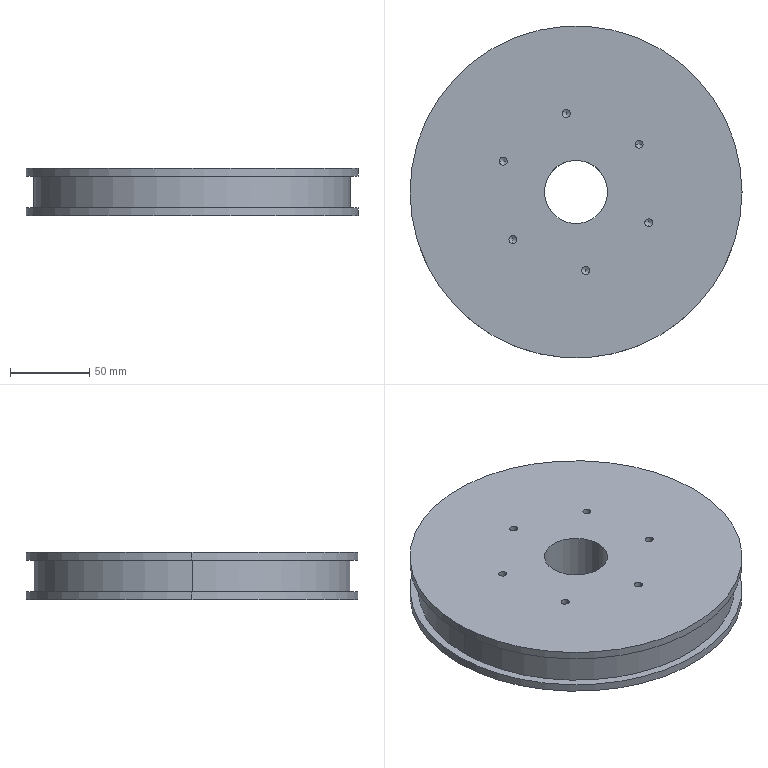Part | SolidWorks | features BaseBody 1 | 1 solid | 36 faces | box 210 x 210 x 30 mm | volume 935154 mm3 | cylinder 20 | cone 12 | plane 4 | commonest cylinder face diameters 5 x12 210 x4 40 x2 200 x2
STEP:
#1=CARTESIAN_POINT('',(-105.,0.,178.202));
#2=VERTEX_POINT('',#1);
#3=CARTESIAN_POINT('',(105.,0.,178.202));
#4=VERTEX_POINT('',#3);
#5=CARTESIAN_POINT('',(0.,0.,178.202));
#6=DIRECTION('',(0.,0.,-1.));
#7=DIRECTION('',(1.,0.,0.));
#8=AXIS2_PLACEMENT_3D('',#5,#6,#7);
#9=CIRCLE('',#8,105.);
#10=EDGE_CURVE('',#2,#4,#9,.T.);
#11=ORIENTED_EDGE('',*,*,#10,.F.);
#12=CARTESIAN_POINT('',(-105.,0.,183.202));
#13=VERTEX_POINT('',#12);
#14=CARTESIAN_POINT('',(-105.,0.,72.202));
#15=DIRECTION('',(0.,0.,1.));
#16=VECTOR('',#15,1000.);
#17=LINE('',#14,#16);
#18=EDGE_CURVE('',#2,#13,#17,.T.);
#19=ORIENTED_EDGE('',*,*,#18,.T.);
#20=CARTESIAN_POINT('',(105.,0.,183.202));
#21=VERTEX_POINT('',#20);
#22=CARTESIAN_POINT('',(0.,0.,183.202));
#23=DIRECTION('',(0.,0.,-1.));
#24=DIRECTION('',(1.,0.,0.));
#25=AXIS2_PLACEMENT_3D('',#22,#23,#24);
#26=CIRCLE('',#25,105.);
#27=EDGE_CURVE('',#13,#21,#26,.T.);
#28=ORIENTED_EDGE('',*,*,#27,.T.);
#29=CARTESIAN_POINT('',(105.,0.,72.202));
#30=DIRECTION('',(0.,0.,1.));
#31=VECTOR('',#30,1000.);
#32=LINE('',#29,#31);
#33=EDGE_CURVE('',#4,#21,#32,.T.);
#34=ORIENTED_EDGE('',*,*,#33,.F.);
#35=EDGE_LOOP('',(#11,#19,#28,#34));
#36=FACE_OUTER_BOUND('',#35,.T.);
#37=CARTESIAN_POINT('',(0.,0.,72.202));
#38=DIRECTION('',(0.,0.,1.));
#39=DIRECTION('',(1.,0.,0.));
#40=AXIS2_PLACEMENT_3D('',#37,#38,#39);
#41=CYLINDRICAL_SURFACE('',#40,105.);
#42=ADVANCED_FACE('',(#36),#41,.T.);
#43=CARTESIAN_POINT('',(-20.,0.,178.202));
#44=VERTEX_POINT('',#43);
#45=CARTESIAN_POINT('',(20.,0.,178.202));
#46=VERTEX_POINT('',#45);
#47=CARTESIAN_POINT('',(0.,0.,178.202));
#48=DIRECTION('',(0.,0.,1.));
#49=DIRECTION('',(1.,0.,0.));
#50=AXIS2_PLACEMENT_3D('',#47,#48,#49);
#51=CIRCLE('',#50,20.);
#52=EDGE_CURVE('',#44,#46,#51,.T.);
#53=ORIENTED_EDGE('',*,*,#52,.F.);
#54=CARTESIAN_POINT('',(-20.,0.,208.202));
#55=VERTEX_POINT('',#54);
#56=CARTESIAN_POINT('',(-20.,0.,177.8));
#57=DIRECTION('',(0.,0.,1.));
#58=VECTOR('',#57,1000.);
#59=LINE('',#56,#58);
#60=EDGE_CURVE('',#44,#55,#59,.T.);
#61=ORIENTED_EDGE('',*,*,#60,.T.);
#62=CARTESIAN_POINT('',(20.,0.,208.202));
#63=VERTEX_POINT('',#62);
#64=CARTESIAN_POINT('',(0.,0.,208.202));
#65=DIRECTION('',(0.,0.,-1.));
#66=DIRECTION('',(1.,0.,0.));
#67=AXIS2_PLACEMENT_3D('',#64,#65,#66);
#68=CIRCLE('',#67,20.);
#69=EDGE_CURVE('',#63,#55,#68,.T.);
#70=ORIENTED_EDGE('',*,*,#69,.F.);
#71=CARTESIAN_POINT('',(20.,0.,177.8));
#72=DIRECTION('',(0.,0.,1.));
#73=VECTOR('',#72,1000.);
#74=LINE('',#71,#73);
#75=EDGE_CURVE('',#46,#63,#74,.T.);
#76=ORIENTED_EDGE('',*,*,#75,.F.);
#77=EDGE_LOOP('',(#53,#61,#70,#76));
#78=FACE_OUTER_BOUND('',#77,.T.);
#79=CARTESIAN_POINT('',(0.,0.,177.8));
#80=DIRECTION('',(0.,0.,1.));
#81=DIRECTION('',(1.,0.,0.));
#82=AXIS2_PLACEMENT_3D('',#79,#80,#81);
#83=CYLINDRICAL_SURFACE('',#82,20.);
#84=ADVANCED_FACE('',(#78),#83,.F.);
#85=CARTESIAN_POINT('',(-100.,0.,203.202));
#86=VERTEX_POINT('',#85);
#87=CARTESIAN_POINT('',(100.,0.,203.202));
#88=VERTEX_POINT('',#87);
#89=CARTESIAN_POINT('',(0.,0.,203.202));
#90=DIRECTION('',(0.,0.,-1.));
#91=DIRECTION('',(-1.,0.,0.));
#92=AXIS2_PLACEMENT_3D('',#89,#90,#91);
#93=CIRCLE('',#92,100.);
#94=EDGE_CURVE('',#86,#88,#93,.T.);
#95=ORIENTED_EDGE('',*,*,#94,.T.);
#96=CARTESIAN_POINT('',(100.,0.,183.202));
#97=VERTEX_POINT('',#96);
#98=CARTESIAN_POINT('',(100.,0.,294.202));
#99=DIRECTION('',(0.,0.,-1.));
#100=VECTOR('',#99,1000.);
#101=LINE('',#98,#100);
#102=EDGE_CURVE('',#88,#97,#101,.T.);
#103=ORIENTED_EDGE('',*,*,#102,.T.);
#104=CARTESIAN_POINT('',(-100.,0.,183.202));
#105=VERTEX_POINT('',#104);
#106=CARTESIAN_POINT('',(0.,0.,183.202));
#107=DIRECTION('',(0.,0.,1.));
#108=DIRECTION('',(-1.,0.,0.));
#109=AXIS2_PLACEMENT_3D('',#106,#107,#108);
#110=CIRCLE('',#109,100.);
#111=EDGE_CURVE('',#97,#105,#110,.T.);
#112=ORIENTED_EDGE('',*,*,#111,.T.);
#113=CARTESIAN_POINT('',(-100.,0.,294.202));
#114=DIRECTION('',(0.,0.,-1.));
#115=VECTOR('',#114,1000.);
#116=LINE('',#113,#115);
#117=EDGE_CURVE('',#86,#105,#116,.T.);
#118=ORIENTED_EDGE('',*,*,#117,.F.);
#119=EDGE_LOOP('',(#95,#103,#112,#118));
#120=FACE_OUTER_BOUND('',#119,.T.);
#121=CARTESIAN_POINT('',(0.,0.,294.202));
#122=DIRECTION('',(0.,0.,-1.));
#123=DIRECTION('',(-1.,0.,0.));
#124=AXIS2_PLACEMENT_3D('',#121,#122,#123);
#125=CYLINDRICAL_SURFACE('',#124,100.);
#126=ADVANCED_FACE('',(#120),#125,.T.);
#127=CARTESIAN_POINT('',(105.,0.,203.202));
#128=VERTEX_POINT('',#127);
#129=CARTESIAN_POINT('',(-105.,0.,203.202));
#130=VERTEX_POINT('',#129);
#131=CARTESIAN_POINT('',(0.,0.,203.202));
#132=DIRECTION('',(0.,0.,1.));
#133=DIRECTION('',(1.,0.,0.));
#134=AXIS2_PLACEMENT_3D('',#131,#132,#133);
#135=CIRCLE('',#134,105.);
#136=EDGE_CURVE('',#128,#130,#135,.T.);
#137=ORIENTED_EDGE('',*,*,#136,.T.);
#138=CARTESIAN_POINT('',(-105.,0.,208.202));
#139=VERTEX_POINT('',#138);
#140=CARTESIAN_POINT('',(-105.,0.,203.202));
#141=DIRECTION('',(0.,0.,1.));
#142=VECTOR('',#141,1000.);
#143=LINE('',#140,#142);
#144=EDGE_CURVE('',#130,#139,#143,.T.);
#145=ORIENTED_EDGE('',*,*,#144,.T.);
#146=CARTESIAN_POINT('',(105.,0.,208.202));
#147=VERTEX_POINT('',#146);
#148=CARTESIAN_POINT('',(0.,0.,208.202));
#149=DIRECTION('',(0.,0.,1.));
#150=DIRECTION('',(1.,0.,0.));
#151=AXIS2_PLACEMENT_3D('',#148,#149,#150);
#152=CIRCLE('',#151,105.);
#153=EDGE_CURVE('',#147,#139,#152,.T.);
#154=ORIENTED_EDGE('',*,*,#153,.F.);
#155=CARTESIAN_POINT('',(105.,0.,203.202));
#156=DIRECTION('',(0.,0.,1.));
#157=VECTOR('',#156,1000.);
#158=LINE('',#155,#157);
#159=EDGE_CURVE('',#128,#147,#158,.T.);
#160=ORIENTED_EDGE('',*,*,#159,.F.);
#161=EDGE_LOOP('',(#137,#145,#154,#160));
#162=FACE_OUTER_BOUND('',#161,.T.);
#163=CARTESIAN_POINT('',(0.,0.,203.202));
#164=DIRECTION('',(0.,0.,1.));
#165=DIRECTION('',(1.,0.,0.));
#166=AXIS2_PLACEMENT_3D('',#163,#164,#165);
#167=CYLINDRICAL_SURFACE('',#166,105.);
#168=ADVANCED_FACE('',(#162),#167,.T.);
#169=CARTESIAN_POINT('',(-8.677,49.617,193.202));
#170=VERTEX_POINT('',#169);
#171=CARTESIAN_POINT('',(-6.177,47.117,193.202));
#172=VERTEX_POINT('',#171);
#173=CARTESIAN_POINT('',(-6.177,49.617,193.202));
#174=DIRECTION('',(0.,0.,1.));
#175=DIRECTION('',(1.,0.,0.));
#176=AXIS2_PLACEMENT_3D('',#173,#174,#175);
#177=CIRCLE('',#176,2.5);
#178=EDGE_CURVE('',#170,#172,#177,.T.);
#179=ORIENTED_EDGE('',*,*,#178,.F.);
#180=CARTESIAN_POINT('',(-8.677,49.617,208.202));
#181=VERTEX_POINT('',#180);
#182=CARTESIAN_POINT('',(-8.677,49.617,208.202));
#183=DIRECTION('',(0.,0.,1.));
#184=VECTOR('',#183,1000.);
#185=LINE('',#182,#184);
#186=EDGE_CURVE('',#170,#181,#185,.T.);
#187=ORIENTED_EDGE('',*,*,#186,.T.);
#188=CARTESIAN_POINT('',(-3.677,49.617,208.202));
#189=VERTEX_POINT('',#188);
#190=CARTESIAN_POINT('',(-6.177,49.617,208.202));
#191=DIRECTION('',(0.,0.,-1.));
#192=DIRECTION('',(1.,0.,0.));
#193=AXIS2_PLACEMENT_3D('',#190,#191,#192);
#194=CIRCLE('',#193,2.5);
#195=EDGE_CURVE('',#189,#181,#194,.T.);
#196=ORIENTED_EDGE('',*,*,#195,.F.);
#197=CARTESIAN_POINT('',(-3.677,49.617,193.202));
#198=VERTEX_POINT('',#197);
#199=CARTESIAN_POINT('',(-3.677,49.617,208.202));
#200=DIRECTION('',(0.,0.,1.));
#201=VECTOR('',#200,1000.);
#202=LINE('',#199,#201);
#203=EDGE_CURVE('',#198,#189,#202,.T.);
#204=ORIENTED_EDGE('',*,*,#203,.F.);
#205=CARTESIAN_POINT('',(-6.177,49.617,193.202));
#206=DIRECTION('',(0.,0.,1.));
#207=DIRECTION('',(1.,0.,0.));
#208=AXIS2_PLACEMENT_3D('',#205,#206,#207);
#209=CIRCLE('',#208,2.5);
#210=EDGE_CURVE('',#172,#198,#209,.T.);
#211=ORIENTED_EDGE('',*,*,#210,.F.);
#212=EDGE_LOOP('',(#179,#187,#196,#204,#211));
#213=FACE_OUTER_BOUND('',#212,.T.);
#214=CARTESIAN_POINT('',(-6.177,49.617,208.202));
#215=DIRECTION('',(0.,0.,1.));
#216=DIRECTION('',(1.,0.,0.));
#217=AXIS2_PLACEMENT_3D('',#214,#215,#216);
#218=CYLINDRICAL_SURFACE('',#217,2.5);
#219=ADVANCED_FACE('',(#213),#218,.F.);
#220=CARTESIAN_POINT('',(-48.558,19.459,193.202));
#221=VERTEX_POINT('',#220);
#222=CARTESIAN_POINT('',(-43.558,19.459,193.202));
#223=VERTEX_POINT('',#222);
#224=CARTESIAN_POINT('',(-46.058,19.459,193.202));
#225=DIRECTION('',(0.,0.,1.));
#226=DIRECTION('',(1.,0.,0.));
#227=AXIS2_PLACEMENT_3D('',#224,#225,#226);
#228=CIRCLE('',#227,2.5);
#229=EDGE_CURVE('',#221,#223,#228,.T.);
#230=ORIENTED_EDGE('',*,*,#229,.F.);
#231=CARTESIAN_POINT('',(-48.558,19.459,208.202));
#232=VERTEX_POINT('',#231);
#233=CARTESIAN_POINT('',(-48.558,19.459,208.202));
#234=DIRECTION('',(0.,0.,1.));
#235=VECTOR('',#234,1000.);
#236=LINE('',#233,#235);
#237=EDGE_CURVE('',#221,#232,#236,.T.);
#238=ORIENTED_EDGE('',*,*,#237,.T.);
#239=CARTESIAN_POINT('',(-43.558,19.459,208.202));
#240=VERTEX_POINT('',#239);
#241=CARTESIAN_POINT('',(-46.058,19.459,208.202));
#242=DIRECTION('',(0.,0.,-1.));
#243=DIRECTION('',(1.,0.,0.));
#244=AXIS2_PLACEMENT_3D('',#241,#242,#243);
#245=CIRCLE('',#244,2.5);
#246=EDGE_CURVE('',#240,#232,#245,.T.);
#247=ORIENTED_EDGE('',*,*,#246,.F.);
#248=CARTESIAN_POINT('',(-43.558,19.459,208.202));
#249=DIRECTION('',(0.,0.,1.));
#250=VECTOR('',#249,1000.);
#251=LINE('',#248,#250);
#252=EDGE_CURVE('',#223,#240,#251,.T.);
#253=ORIENTED_EDGE('',*,*,#252,.F.);
#254=EDGE_LOOP('',(#230,#238,#247,#253));
#255=FACE_OUTER_BOUND('',#254,.T.);
#256=CARTESIAN_POINT('',(-46.058,19.459,208.202));
#257=DIRECTION('',(0.,0.,1.));
#258=DIRECTION('',(1.,0.,0.));
#259=AXIS2_PLACEMENT_3D('',#256,#257,#258);
#260=CYLINDRICAL_SURFACE('',#259,2.5);
#261=ADVANCED_FACE('',(#255),#260,.F.);
#262=CARTESIAN_POINT('',(-42.381,-30.158,193.202));
#263=VERTEX_POINT('',#262);
#264=CARTESIAN_POINT('',(-39.881,-32.658,193.202));
#265=VERTEX_POINT('',#264);
#266=CARTESIAN_POINT('',(-39.881,-30.158,193.202));
#267=DIRECTION('',(0.,0.,1.));
#268=DIRECTION('',(1.,0.,0.));
#269=AXIS2_PLACEMENT_3D('',#266,#267,#268);
#270=CIRCLE('',#269,2.5);
#271=EDGE_CURVE('',#263,#265,#270,.T.);
#272=ORIENTED_EDGE('',*,*,#271,.F.);
#273=CARTESIAN_POINT('',(-42.381,-30.158,208.202));
#274=VERTEX_POINT('',#273);
#275=CARTESIAN_POINT('',(-42.381,-30.158,208.202));
#276=DIRECTION('',(0.,0.,1.));
#277=VECTOR('',#276,1000.);
#278=LINE('',#275,#277);
#279=EDGE_CURVE('',#263,#274,#278,.T.);
#280=ORIENTED_EDGE('',*,*,#279,.T.);
#281=CARTESIAN_POINT('',(-37.381,-30.158,208.202));
#282=VERTEX_POINT('',#281);
#283=CARTESIAN_POINT('',(-39.881,-30.158,208.202));
#284=DIRECTION('',(0.,0.,-1.));
#285=DIRECTION('',(1.,0.,0.));
#286=AXIS2_PLACEMENT_3D('',#283,#284,#285);
#287=CIRCLE('',#286,2.5);
#288=EDGE_CURVE('',#282,#274,#287,.T.);
#289=ORIENTED_EDGE('',*,*,#288,.F.);
#290=CARTESIAN_POINT('',(-37.381,-30.158,193.202));
#291=VERTEX_POINT('',#290);
#292=CARTESIAN_POINT('',(-37.381,-30.158,208.202));
#293=DIRECTION('',(0.,0.,1.));
#294=VECTOR('',#293,1000.);
#295=LINE('',#292,#294);
#296=EDGE_CURVE('',#291,#282,#295,.T.);
#297=ORIENTED_EDGE('',*,*,#296,.F.);
#298=CARTESIAN_POINT('',(-39.881,-30.158,193.202));
#299=DIRECTION('',(0.,0.,1.));
#300=DIRECTION('',(1.,0.,0.));
#301=AXIS2_PLACEMENT_3D('',#298,#299,#300);
#302=CIRCLE('',#301,2.5);
#303=EDGE_CURVE('',#265,#291,#302,.T.);
#304=ORIENTED_EDGE('',*,*,#303,.F.);
#305=EDGE_LOOP('',(#272,#280,#289,#297,#304));
#306=FACE_OUTER_BOUND('',#305,.T.);
#307=CARTESIAN_POINT('',(-39.881,-30.158,208.202));
#308=DIRECTION('',(0.,0.,1.));
#309=DIRECTION('',(1.,0.,0.));
#310=AXIS2_PLACEMENT_3D('',#307,#308,#309);
#311=CYLINDRICAL_SURFACE('',#310,2.5);
#312=ADVANCED_FACE('',(#306),#311,.F.);
#313=CARTESIAN_POINT('',(3.677,-49.617,193.202));
#314=VERTEX_POINT('',#313);
#315=CARTESIAN_POINT('',(6.177,-52.117,193.202));
#316=VERTEX_POINT('',#315);
#317=CARTESIAN_POINT('',(6.177,-49.617,193.202));
#318=DIRECTION('',(0.,0.,1.));
#319=DIRECTION('',(1.,0.,0.));
#320=AXIS2_PLACEMENT_3D('',#317,#318,#319);
#321=CIRCLE('',#320,2.5);
#322=EDGE_CURVE('',#314,#316,#321,.T.);
#323=ORIENTED_EDGE('',*,*,#322,.F.);
#324=CARTESIAN_POINT('',(3.677,-49.617,208.202));
#325=VERTEX_POINT('',#324);
#326=CARTESIAN_POINT('',(3.677,-49.617,208.202));
#327=DIRECTION('',(0.,0.,1.));
#328=VECTOR('',#327,1000.);
#329=LINE('',#326,#328);
#330=EDGE_CURVE('',#314,#325,#329,.T.);
#331=ORIENTED_EDGE('',*,*,#330,.T.);
#332=CARTESIAN_POINT('',(8.677,-49.617,208.202));
#333=VERTEX_POINT('',#332);
#334=CARTESIAN_POINT('',(6.177,-49.617,208.202));
#335=DIRECTION('',(0.,0.,-1.));
#336=DIRECTION('',(1.,0.,0.));
#337=AXIS2_PLACEMENT_3D('',#334,#335,#336);
#338=CIRCLE('',#337,2.5);
#339=EDGE_CURVE('',#333,#325,#338,.T.);
#340=ORIENTED_EDGE('',*,*,#339,.F.);
#341=CARTESIAN_POINT('',(8.677,-49.617,193.202));
#342=VERTEX_POINT('',#341);
#343=CARTESIAN_POINT('',(8.677,-49.617,208.202));
#344=DIRECTION('',(0.,0.,1.));
#345=VECTOR('',#344,1000.);
#346=LINE('',#343,#345);
#347=EDGE_CURVE('',#342,#333,#346,.T.);
#348=ORIENTED_EDGE('',*,*,#347,.F.);
#349=CARTESIAN_POINT('',(6.177,-49.617,193.202));
#350=DIRECTION('',(0.,0.,1.));
#351=DIRECTION('',(1.,0.,0.));
#352=AXIS2_PLACEMENT_3D('',#349,#350,#351);
#353=CIRCLE('',#352,2.5);
#354=EDGE_CURVE('',#316,#342,#353,.T.);
#355=ORIENTED_EDGE('',*,*,#354,.F.);
#356=EDGE_LOOP('',(#323,#331,#340,#348,#355));
#357=FACE_OUTER_BOUND('',#356,.T.);
#358=CARTESIAN_POINT('',(6.177,-49.617,208.202));
#359=DIRECTION('',(0.,0.,1.));
#360=DIRECTION('',(1.,0.,0.));
#361=AXIS2_PLACEMENT_3D('',#358,#359,#360);
#362=CYLINDRICAL_SURFACE('',#361,2.5);
#363=ADVANCED_FACE('',(#357),#362,.F.);
#364=CARTESIAN_POINT('',(43.558,-19.459,193.202));
#365=VERTEX_POINT('',#364);
#366=CARTESIAN_POINT('',(46.058,-21.959,193.202));
#367=VERTEX_POINT('',#366);
#368=CARTESIAN_POINT('',(46.058,-19.459,193.202));
#369=DIRECTION('',(0.,0.,1.));
#370=DIRECTION('',(1.,0.,0.));
#371=AXIS2_PLACEMENT_3D('',#368,#369,#370);
#372=CIRCLE('',#371,2.5);
#373=EDGE_CURVE('',#365,#367,#372,.T.);
#374=ORIENTED_EDGE('',*,*,#373,.F.);
#375=CARTESIAN_POINT('',(43.558,-19.459,208.202));
#376=VERTEX_POINT('',#375);
#377=CARTESIAN_POINT('',(43.558,-19.459,208.202));
#378=DIRECTION('',(0.,0.,1.));
#379=VECTOR('',#378,1000.);
#380=LINE('',#377,#379);
#381=EDGE_CURVE('',#365,#376,#380,.T.);
#382=ORIENTED_EDGE('',*,*,#381,.T.);
#383=CARTESIAN_POINT('',(48.558,-19.459,208.202));
#384=VERTEX_POINT('',#383);
#385=CARTESIAN_POINT('',(46.058,-19.459,208.202));
#386=DIRECTION('',(0.,0.,-1.));
#387=DIRECTION('',(1.,0.,0.));
#388=AXIS2_PLACEMENT_3D('',#385,#386,#387);
#389=CIRCLE('',#388,2.5);
#390=EDGE_CURVE('',#384,#376,#389,.T.);
#391=ORIENTED_EDGE('',*,*,#390,.F.);
#392=CARTESIAN_POINT('',(48.558,-19.459,193.202));
#393=VERTEX_POINT('',#392);
#394=CARTESIAN_POINT('',(48.558,-19.459,208.202));
#395=DIRECTION('',(0.,0.,1.));
#396=VECTOR('',#395,1000.);
#397=LINE('',#394,#396);
#398=EDGE_CURVE('',#393,#384,#397,.T.);
#399=ORIENTED_EDGE('',*,*,#398,.F.);
#400=CARTESIAN_POINT('',(46.058,-19.459,193.202));
#401=DIRECTION('',(0.,0.,1.));
#402=DIRECTION('',(1.,0.,0.));
#403=AXIS2_PLACEMENT_3D('',#400,#401,#402);
#404=CIRCLE('',#403,2.5);
#405=EDGE_CURVE('',#367,#393,#404,.T.);
#406=ORIENTED_EDGE('',*,*,#405,.F.);
#407=EDGE_LOOP('',(#374,#382,#391,#399,#406));
#408=FACE_OUTER_BOUND('',#407,.T.);
#409=CARTESIAN_POINT('',(46.058,-19.459,208.202));
#410=DIRECTION('',(0.,0.,1.));
#411=DIRECTION('',(1.,0.,0.));
#412=AXIS2_PLACEMENT_3D('',#409,#410,#411);
#413=CYLINDRICAL_SURFACE('',#412,2.5);
#414=ADVANCED_FACE('',(#408),#413,.F.);
#415=CARTESIAN_POINT('',(37.381,30.158,193.202));
#416=VERTEX_POINT('',#415);
#417=CARTESIAN_POINT('',(42.381,30.158,193.202));
#418=VERTEX_POINT('',#417);
#419=CARTESIAN_POINT('',(39.881,30.158,193.202));
#420=DIRECTION('',(0.,0.,1.));
#421=DIRECTION('',(1.,0.,0.));
#422=AXIS2_PLACEMENT_3D('',#419,#420,#421);
#423=CIRCLE('',#422,2.5);
#424=EDGE_CURVE('',#416,#418,#423,.T.);
#425=ORIENTED_EDGE('',*,*,#424,.F.);
#426=CARTESIAN_POINT('',(37.381,30.158,208.202));
#427=VERTEX_POINT('',#426);
#428=CARTESIAN_POINT('',(37.381,30.158,208.202));
#429=DIRECTION('',(0.,0.,1.));
#430=VECTOR('',#429,1000.);
#431=LINE('',#428,#430);
#432=EDGE_CURVE('',#416,#427,#431,.T.);
#433=ORIENTED_EDGE('',*,*,#432,.T.);
#434=CARTESIAN_POINT('',(42.381,30.158,208.202));
#435=VERTEX_POINT('',#434);
#436=CARTESIAN_POINT('',(39.881,30.158,208.202));
#437=DIRECTION('',(0.,0.,-1.));
#438=DIRECTION('',(1.,0.,0.));
#439=AXIS2_PLACEMENT_3D('',#436,#437,#438);
#440=CIRCLE('',#439,2.5);
#441=EDGE_CURVE('',#435,#427,#440,.T.);
#442=ORIENTED_EDGE('',*,*,#441,.F.);
#443=CARTESIAN_POINT('',(42.381,30.158,208.202));
#444=DIRECTION('',(0.,0.,1.));
#445=VECTOR('',#444,1000.);
#446=LINE('',#443,#445);
#447=EDGE_CURVE('',#418,#435,#446,.T.);
#448=ORIENTED_EDGE('',*,*,#447,.F.);
#449=EDGE_LOOP('',(#425,#433,#442,#448));
#450=FACE_OUTER_BOUND('',#449,.T.);
#451=CARTESIAN_POINT('',(39.881,30.158,208.202));
#452=DIRECTION('',(0.,0.,1.));
#453=DIRECTION('',(1.,0.,0.));
#454=AXIS2_PLACEMENT_3D('',#451,#452,#453);
#455=CYLINDRICAL_SURFACE('',#454,2.5);
#456=ADVANCED_FACE('',(#450),#455,.F.);
#457=CARTESIAN_POINT('',(-6.177,49.617,191.7));
#458=VERTEX_POINT('',#457);
#459=CARTESIAN_POINT('',(-6.177,47.117,193.202));
#460=DIRECTION('',(0.,-0.8572,0.515));
#461=VECTOR('',#460,1000.);
#462=LINE('',#459,#461);
#463=EDGE_CURVE('',#458,#172,#462,.T.);
#464=ORIENTED_EDGE('',*,*,#463,.F.);
#465=CARTESIAN_POINT('',(-6.177,52.117,193.202));
#466=VERTEX_POINT('',#465);
#467=CARTESIAN_POINT('',(-6.177,52.117,193.202));
#468=DIRECTION('',(0.,0.8572,0.515));
#469=VECTOR('',#468,1000.);
#470=LINE('',#467,#469);
#471=EDGE_CURVE('',#458,#466,#470,.T.);
#472=ORIENTED_EDGE('',*,*,#471,.T.);
#473=CARTESIAN_POINT('',(-6.177,49.617,193.202));
#474=DIRECTION('',(0.,0.,1.));
#475=DIRECTION('',(1.,0.,0.));
#476=AXIS2_PLACEMENT_3D('',#473,#474,#475);
#477=CIRCLE('',#476,2.5);
#478=EDGE_CURVE('',#466,#170,#477,.T.);
#479=ORIENTED_EDGE('',*,*,#478,.T.);
#480=ORIENTED_EDGE('',*,*,#178,.T.);
#481=EDGE_LOOP('',(#464,#472,#479,#480));
#482=FACE_OUTER_BOUND('',#481,.T.);
#483=CARTESIAN_POINT('',(-6.177,49.617,193.202));
#484=DIRECTION('',(0.,0.,1.));
#485=DIRECTION('',(0.,-1.,0.));
#486=AXIS2_PLACEMENT_3D('',#483,#484,#485);
#487=CONICAL_SURFACE('',#486,2.5,1.03);
#488=ADVANCED_FACE('',(#482),#487,.F.);
#489=CARTESIAN_POINT('',(-46.058,19.459,191.7));
#490=VERTEX_POINT('',#489);
#491=CARTESIAN_POINT('',(-43.558,19.459,193.202));
#492=DIRECTION('',(0.8572,0.,0.515));
#493=VECTOR('',#492,1000.);
#494=LINE('',#491,#493);
#495=EDGE_CURVE('',#490,#223,#494,.T.);
#496=ORIENTED_EDGE('',*,*,#495,.F.);
#497=CARTESIAN_POINT('',(-48.558,19.459,193.202));
#498=DIRECTION('',(-0.8572,0.,0.515));
#499=VECTOR('',#498,1000.);
#500=LINE('',#497,#499);
#501=EDGE_CURVE('',#490,#221,#500,.T.);
#502=ORIENTED_EDGE('',*,*,#501,.T.);
#503=ORIENTED_EDGE('',*,*,#229,.T.);
#504=EDGE_LOOP('',(#496,#502,#503));
#505=FACE_OUTER_BOUND('',#504,.T.);
#506=CARTESIAN_POINT('',(-46.058,19.459,193.202));
#507=DIRECTION('',(0.,0.,1.));
#508=DIRECTION('',(1.,0.,0.));
#509=AXIS2_PLACEMENT_3D('',#506,#507,#508);
#510=CONICAL_SURFACE('',#509,2.5,1.03);
#511=ADVANCED_FACE('',(#505),#510,.F.);
#512=CARTESIAN_POINT('',(-39.881,-30.158,191.7));
#513=VERTEX_POINT('',#512);
#514=CARTESIAN_POINT('',(-39.881,-32.658,193.202));
#515=DIRECTION('',(0.,-0.8572,0.515));
#516=VECTOR('',#515,1000.);
#517=LINE('',#514,#516);
#518=EDGE_CURVE('',#513,#265,#517,.T.);
#519=ORIENTED_EDGE('',*,*,#518,.F.);
#520=CARTESIAN_POINT('',(-39.881,-27.658,193.202));
#521=VERTEX_POINT('',#520);
#522=CARTESIAN_POINT('',(-39.881,-27.658,193.202));
#523=DIRECTION('',(0.,0.8572,0.515));
#524=VECTOR('',#523,1000.);
#525=LINE('',#522,#524);
#526=EDGE_CURVE('',#513,#521,#525,.T.);
#527=ORIENTED_EDGE('',*,*,#526,.T.);
#528=CARTESIAN_POINT('',(-39.881,-30.158,193.202));
#529=DIRECTION('',(0.,0.,1.));
#530=DIRECTION('',(1.,0.,0.));
#531=AXIS2_PLACEMENT_3D('',#528,#529,#530);
#532=CIRCLE('',#531,2.5);
#533=EDGE_CURVE('',#521,#263,#532,.T.);
#534=ORIENTED_EDGE('',*,*,#533,.T.);
#535=ORIENTED_EDGE('',*,*,#271,.T.);
#536=EDGE_LOOP('',(#519,#527,#534,#535));
#537=FACE_OUTER_BOUND('',#536,.T.);
#538=CARTESIAN_POINT('',(-39.881,-30.158,193.202));
#539=DIRECTION('',(0.,0.,1.));
#540=DIRECTION('',(0.,-1.,0.));
#541=AXIS2_PLACEMENT_3D('',#538,#539,#540);
#542=CONICAL_SURFACE('',#541,2.5,1.03);
#543=ADVANCED_FACE('',(#537),#542,.F.);
#544=CARTESIAN_POINT('',(6.177,-49.617,191.7));
#545=VERTEX_POINT('',#544);
#546=CARTESIAN_POINT('',(6.177,-52.117,193.202));
#547=DIRECTION('',(0.,-0.8572,0.515));
#548=VECTOR('',#547,1000.);
#549=LINE('',#546,#548);
#550=EDGE_CURVE('',#545,#316,#549,.T.);
#551=ORIENTED_EDGE('',*,*,#550,.F.);
#552=CARTESIAN_POINT('',(6.177,-47.117,193.202));
#553=VERTEX_POINT('',#552);
#554=CARTESIAN_POINT('',(6.177,-47.117,193.202));
#555=DIRECTION('',(0.,0.8572,0.515));
#556=VECTOR('',#555,1000.);
#557=LINE('',#554,#556);
#558=EDGE_CURVE('',#545,#553,#557,.T.);
#559=ORIENTED_EDGE('',*,*,#558,.T.);
#560=CARTESIAN_POINT('',(6.177,-49.617,193.202));
#561=DIRECTION('',(0.,0.,1.));
#562=DIRECTION('',(1.,0.,0.));
#563=AXIS2_PLACEMENT_3D('',#560,#561,#562);
#564=CIRCLE('',#563,2.5);
#565=EDGE_CURVE('',#553,#314,#564,.T.);
#566=ORIENTED_EDGE('',*,*,#565,.T.);
#567=ORIENTED_EDGE('',*,*,#322,.T.);
#568=EDGE_LOOP('',(#551,#559,#566,#567));
#569=FACE_OUTER_BOUND('',#568,.T.);
#570=CARTESIAN_POINT('',(6.177,-49.617,193.202));
#571=DIRECTION('',(0.,0.,1.));
#572=DIRECTION('',(0.,-1.,0.));
#573=AXIS2_PLACEMENT_3D('',#570,#571,#572);
#574=CONICAL_SURFACE('',#573,2.5,1.03);
#575=ADVANCED_FACE('',(#569),#574,.F.);
#576=CARTESIAN_POINT('',(46.058,-19.459,191.7));
#577=VERTEX_POINT('',#576);
#578=CARTESIAN_POINT('',(46.058,-21.959,193.202));
#579=DIRECTION('',(0.,-0.8572,0.515));
#580=VECTOR('',#579,1000.);
#581=LINE('',#578,#580);
#582=EDGE_CURVE('',#577,#367,#581,.T.);
#583=ORIENTED_EDGE('',*,*,#582,.F.);
#584=CARTESIAN_POINT('',(46.058,-16.959,193.202));
#585=VERTEX_POINT('',#584);
#586=CARTESIAN_POINT('',(46.058,-16.959,193.202));
#587=DIRECTION('',(0.,0.8572,0.515));
#588=VECTOR('',#587,1000.);
#589=LINE('',#586,#588);
#590=EDGE_CURVE('',#577,#585,#589,.T.);
#591=ORIENTED_EDGE('',*,*,#590,.T.);
#592=CARTESIAN_POINT('',(46.058,-19.459,193.202));
#593=DIRECTION('',(0.,0.,1.));
#594=DIRECTION('',(1.,0.,0.));
#595=AXIS2_PLACEMENT_3D('',#592,#593,#594);
#596=CIRCLE('',#595,2.5);
#597=EDGE_CURVE('',#585,#365,#596,.T.);
#598=ORIENTED_EDGE('',*,*,#597,.T.);
#599=ORIENTED_EDGE('',*,*,#373,.T.);
#600=EDGE_LOOP('',(#583,#591,#598,#599));
#601=FACE_OUTER_BOUND('',#600,.T.);
#602=CARTESIAN_POINT('',(46.058,-19.459,193.202));
#603=DIRECTION('',(0.,0.,1.));
#604=DIRECTION('',(0.,-1.,0.));
#605=AXIS2_PLACEMENT_3D('',#602,#603,#604);
#606=CONICAL_SURFACE('',#605,2.5,1.03);
#607=ADVANCED_FACE('',(#601),#606,.F.);
#608=CARTESIAN_POINT('',(39.881,30.158,191.7));
#609=VERTEX_POINT('',#608);
#610=CARTESIAN_POINT('',(42.381,30.158,193.202));
#611=DIRECTION('',(0.8572,0.,0.515));
#612=VECTOR('',#611,1000.);
#613=LINE('',#610,#612);
#614=EDGE_CURVE('',#609,#418,#613,.T.);
#615=ORIENTED_EDGE('',*,*,#614,.F.);
#616=CARTESIAN_POINT('',(37.381,30.158,193.202));
#617=DIRECTION('',(-0.8572,0.,0.515));
#618=VECTOR('',#617,1000.);
#619=LINE('',#616,#618);
#620=EDGE_CURVE('',#609,#416,#619,.T.);
#621=ORIENTED_EDGE('',*,*,#620,.T.);
#622=ORIENTED_EDGE('',*,*,#424,.T.);
#623=EDGE_LOOP('',(#615,#621,#622));
#624=FACE_OUTER_BOUND('',#623,.T.);
#625=CARTESIAN_POINT('',(39.881,30.158,193.202));
#626=DIRECTION('',(0.,0.,1.));
#627=DIRECTION('',(1.,0.,0.));
#628=AXIS2_PLACEMENT_3D('',#625,#626,#627);
#629=CONICAL_SURFACE('',#628,2.5,1.03);
#630=ADVANCED_FACE('',(#624),#629,.F.);
#631=CARTESIAN_POINT('',(0.,0.,178.202));
#632=DIRECTION('',(0.,0.,-1.));
#633=DIRECTION('',(1.,0.,0.));
#634=AXIS2_PLACEMENT_3D('',#631,#632,#633);
#635=CIRCLE('',#634,105.);
#636=EDGE_CURVE('',#4,#2,#635,.T.);
#637=ORIENTED_EDGE('',*,*,#636,.T.);
#638=ORIENTED_EDGE('',*,*,#10,.T.);
#639=EDGE_LOOP('',(#637,#638));
#640=FACE_OUTER_BOUND('',#639,.T.);
#641=CARTESIAN_POINT('',(0.,0.,178.202));
#642=DIRECTION('',(0.,0.,1.));
#643=DIRECTION('',(1.,0.,0.));
#644=AXIS2_PLACEMENT_3D('',#641,#642,#643);
#645=CIRCLE('',#644,20.);
#646=EDGE_CURVE('',#46,#44,#645,.T.);
#647=ORIENTED_EDGE('',*,*,#646,.T.);
#648=ORIENTED_EDGE('',*,*,#52,.T.);
#649=EDGE_LOOP('',(#647,#648));
#650=FACE_BOUND('',#649,.T.);
#651=CARTESIAN_POINT('',(-431.187,336.743,178.202));
#652=DIRECTION('',(0.,0.,-1.));
#653=DIRECTION('',(0.,1.,0.));
#654=AXIS2_PLACEMENT_3D('',#651,#652,#653);
#655=PLANE('',#654);
#656=ADVANCED_FACE('',(#640,#650),#655,.T.);
#657=ORIENTED_EDGE('',*,*,#18,.F.);
#658=ORIENTED_EDGE('',*,*,#636,.F.);
#659=ORIENTED_EDGE('',*,*,#33,.T.);
#660=CARTESIAN_POINT('',(0.,0.,183.202));
#661=DIRECTION('',(0.,0.,-1.));
#662=DIRECTION('',(1.,0.,0.));
#663=AXIS2_PLACEMENT_3D('',#660,#661,#662);
#664=CIRCLE('',#663,105.);
#665=EDGE_CURVE('',#21,#13,#664,.T.);
#666=ORIENTED_EDGE('',*,*,#665,.T.);
#667=EDGE_LOOP('',(#657,#658,#659,#666));
#668=FACE_OUTER_BOUND('',#667,.T.);
#669=CARTESIAN_POINT('',(0.,0.,72.202));
#670=DIRECTION('',(0.,0.,1.));
#671=DIRECTION('',(1.,0.,0.));
#672=AXIS2_PLACEMENT_3D('',#669,#670,#671);
#673=CYLINDRICAL_SURFACE('',#672,105.);
#674=ADVANCED_FACE('',(#668),#673,.T.);
#675=ORIENTED_EDGE('',*,*,#60,.F.);
#676=ORIENTED_EDGE('',*,*,#646,.F.);
#677=ORIENTED_EDGE('',*,*,#75,.T.);
#678=CARTESIAN_POINT('',(0.,0.,208.202));
#679=DIRECTION('',(0.,0.,-1.));
#680=DIRECTION('',(1.,0.,0.));
#681=AXIS2_PLACEMENT_3D('',#678,#679,#680);
#682=CIRCLE('',#681,20.);
#683=EDGE_CURVE('',#55,#63,#682,.T.);
#684=ORIENTED_EDGE('',*,*,#683,.F.);
#685=EDGE_LOOP('',(#675,#676,#677,#684));
#686=FACE_OUTER_BOUND('',#685,.T.);
#687=CARTESIAN_POINT('',(0.,0.,177.8));
#688=DIRECTION('',(0.,0.,1.));
#689=DIRECTION('',(1.,0.,0.));
#690=AXIS2_PLACEMENT_3D('',#687,#688,#689);
#691=CYLINDRICAL_SURFACE('',#690,20.);
#692=ADVANCED_FACE('',(#686),#691,.F.);
#693=ORIENTED_EDGE('',*,*,#665,.F.);
#694=ORIENTED_EDGE('',*,*,#27,.F.);
#695=EDGE_LOOP('',(#693,#694));
#696=FACE_OUTER_BOUND('',#695,.T.);
#697=CARTESIAN_POINT('',(0.,0.,183.202));
#698=DIRECTION('',(0.,0.,1.));
#699=DIRECTION('',(-1.,0.,0.));
#700=AXIS2_PLACEMENT_3D('',#697,#698,#699);
#701=CIRCLE('',#700,100.);
#702=EDGE_CURVE('',#105,#97,#701,.T.);
#703=ORIENTED_EDGE('',*,*,#702,.F.);
#704=ORIENTED_EDGE('',*,*,#111,.F.);
#705=EDGE_LOOP('',(#703,#704));
#706=FACE_BOUND('',#705,.T.);
#707=CARTESIAN_POINT('',(-431.187,336.743,183.202));
#708=DIRECTION('',(0.,0.,-1.));
#709=DIRECTION('',(0.,1.,0.));
#710=AXIS2_PLACEMENT_3D('',#707,#708,#709);
#711=PLANE('',#710);
#712=ADVANCED_FACE('',(#696,#706),#711,.F.);
#713=ORIENTED_EDGE('',*,*,#153,.T.);
#714=CARTESIAN_POINT('',(0.,0.,208.202));
#715=DIRECTION('',(0.,0.,1.));
#716=DIRECTION('',(1.,0.,0.));
#717=AXIS2_PLACEMENT_3D('',#714,#715,#716);
#718=CIRCLE('',#717,105.);
#719=EDGE_CURVE('',#139,#147,#718,.T.);
#720=ORIENTED_EDGE('',*,*,#719,.T.);
#721=EDGE_LOOP('',(#713,#720));
#722=FACE_OUTER_BOUND('',#721,.T.);
#723=ORIENTED_EDGE('',*,*,#69,.T.);
#724=ORIENTED_EDGE('',*,*,#683,.T.);
#725=EDGE_LOOP('',(#723,#724));
#726=FACE_BOUND('',#725,.T.);
#727=ORIENTED_EDGE('',*,*,#195,.T.);
#728=CARTESIAN_POINT('',(-6.177,49.617,208.202));
#729=DIRECTION('',(0.,0.,-1.));
#730=DIRECTION('',(1.,0.,0.));
#731=AXIS2_PLACEMENT_3D('',#728,#729,#730);
#732=CIRCLE('',#731,2.5);
#733=EDGE_CURVE('',#181,#189,#732,.T.);
#734=ORIENTED_EDGE('',*,*,#733,.T.);
#735=EDGE_LOOP('',(#727,#734));
#736=FACE_BOUND('',#735,.T.);
#737=ORIENTED_EDGE('',*,*,#246,.T.);
#738=CARTESIAN_POINT('',(-46.058,19.459,208.202));
#739=DIRECTION('',(0.,0.,-1.));
#740=DIRECTION('',(1.,0.,0.));
#741=AXIS2_PLACEMENT_3D('',#738,#739,#740);
#742=CIRCLE('',#741,2.5);
#743=EDGE_CURVE('',#232,#240,#742,.T.);
#744=ORIENTED_EDGE('',*,*,#743,.T.);
#745=EDGE_LOOP('',(#737,#744));
#746=FACE_BOUND('',#745,.T.);
#747=ORIENTED_EDGE('',*,*,#288,.T.);
#748=CARTESIAN_POINT('',(-39.881,-30.158,208.202));
#749=DIRECTION('',(0.,0.,-1.));
#750=DIRECTION('',(1.,0.,0.));
#751=AXIS2_PLACEMENT_3D('',#748,#749,#750);
#752=CIRCLE('',#751,2.5);
#753=EDGE_CURVE('',#274,#282,#752,.T.);
#754=ORIENTED_EDGE('',*,*,#753,.T.);
#755=EDGE_LOOP('',(#747,#754));
#756=FACE_BOUND('',#755,.T.);
#757=ORIENTED_EDGE('',*,*,#339,.T.);
#758=CARTESIAN_POINT('',(6.177,-49.617,208.202));
#759=DIRECTION('',(0.,0.,-1.));
#760=DIRECTION('',(1.,0.,0.));
#761=AXIS2_PLACEMENT_3D('',#758,#759,#760);
#762=CIRCLE('',#761,2.5);
#763=EDGE_CURVE('',#325,#333,#762,.T.);
#764=ORIENTED_EDGE('',*,*,#763,.T.);
#765=EDGE_LOOP('',(#757,#764));
#766=FACE_BOUND('',#765,.T.);
#767=ORIENTED_EDGE('',*,*,#390,.T.);
#768=CARTESIAN_POINT('',(46.058,-19.459,208.202));
#769=DIRECTION('',(0.,0.,-1.));
#770=DIRECTION('',(1.,0.,0.));
#771=AXIS2_PLACEMENT_3D('',#768,#769,#770);
#772=CIRCLE('',#771,2.5);
#773=EDGE_CURVE('',#376,#384,#772,.T.);
#774=ORIENTED_EDGE('',*,*,#773,.T.);
#775=EDGE_LOOP('',(#767,#774));
#776=FACE_BOUND('',#775,.T.);
#777=ORIENTED_EDGE('',*,*,#441,.T.);
#778=CARTESIAN_POINT('',(39.881,30.158,208.202));
#779=DIRECTION('',(0.,0.,-1.));
#780=DIRECTION('',(1.,0.,0.));
#781=AXIS2_PLACEMENT_3D('',#778,#779,#780);
#782=CIRCLE('',#781,2.5);
#783=EDGE_CURVE('',#427,#435,#782,.T.);
#784=ORIENTED_EDGE('',*,*,#783,.T.);
#785=EDGE_LOOP('',(#777,#784));
#786=FACE_BOUND('',#785,.T.);
#787=CARTESIAN_POINT('',(-431.187,336.743,208.202));
#788=DIRECTION('',(0.,0.,1.));
#789=DIRECTION('',(0.,-1.,0.));
#790=AXIS2_PLACEMENT_3D('',#787,#788,#789);
#791=PLANE('',#790);
#792=ADVANCED_FACE('',(#722,#726,#736,#746,#756,#766,#776,#786),#791,.T.);
#793=ORIENTED_EDGE('',*,*,#102,.F.);
#794=CARTESIAN_POINT('',(0.,0.,203.202));
#795=DIRECTION('',(0.,0.,-1.));
#796=DIRECTION('',(-1.,0.,0.));
#797=AXIS2_PLACEMENT_3D('',#794,#795,#796);
#798=CIRCLE('',#797,100.);
#799=EDGE_CURVE('',#88,#86,#798,.T.);
#800=ORIENTED_EDGE('',*,*,#799,.T.);
#801=ORIENTED_EDGE('',*,*,#117,.T.);
#802=ORIENTED_EDGE('',*,*,#702,.T.);
#803=EDGE_LOOP('',(#793,#800,#801,#802));
#804=FACE_OUTER_BOUND('',#803,.T.);
#805=CARTESIAN_POINT('',(0.,0.,294.202));
#806=DIRECTION('',(0.,0.,-1.));
#807=DIRECTION('',(-1.,0.,0.));
#808=AXIS2_PLACEMENT_3D('',#805,#806,#807);
#809=CYLINDRICAL_SURFACE('',#808,100.);
#810=ADVANCED_FACE('',(#804),#809,.T.);
#811=ORIENTED_EDGE('',*,*,#144,.F.);
#812=CARTESIAN_POINT('',(0.,0.,203.202));
#813=DIRECTION('',(0.,0.,1.));
#814=DIRECTION('',(1.,0.,0.));
#815=AXIS2_PLACEMENT_3D('',#812,#813,#814);
#816=CIRCLE('',#815,105.);
#817=EDGE_CURVE('',#130,#128,#816,.T.);
#818=ORIENTED_EDGE('',*,*,#817,.T.);
#819=ORIENTED_EDGE('',*,*,#159,.T.);
#820=ORIENTED_EDGE('',*,*,#719,.F.);
#821=EDGE_LOOP('',(#811,#818,#819,#820));
#822=FACE_OUTER_BOUND('',#821,.T.);
#823=CARTESIAN_POINT('',(0.,0.,203.202));
#824=DIRECTION('',(0.,0.,1.));
#825=DIRECTION('',(1.,0.,0.));
#826=AXIS2_PLACEMENT_3D('',#823,#824,#825);
#827=CYLINDRICAL_SURFACE('',#826,105.);
#828=ADVANCED_FACE('',(#822),#827,.T.);
#829=ORIENTED_EDGE('',*,*,#186,.F.);
#830=ORIENTED_EDGE('',*,*,#478,.F.);
#831=CARTESIAN_POINT('',(-6.177,49.617,193.202));
#832=DIRECTION('',(0.,0.,1.));
#833=DIRECTION('',(1.,0.,0.));
#834=AXIS2_PLACEMENT_3D('',#831,#832,#833);
#835=CIRCLE('',#834,2.5);
#836=EDGE_CURVE('',#198,#466,#835,.T.);
#837=ORIENTED_EDGE('',*,*,#836,.F.);
#838=ORIENTED_EDGE('',*,*,#203,.T.);
#839=ORIENTED_EDGE('',*,*,#733,.F.);
#840=EDGE_LOOP('',(#829,#830,#837,#838,#839));
#841=FACE_OUTER_BOUND('',#840,.T.);
#842=CARTESIAN_POINT('',(-6.177,49.617,208.202));
#843=DIRECTION('',(0.,0.,1.));
#844=DIRECTION('',(1.,0.,0.));
#845=AXIS2_PLACEMENT_3D('',#842,#843,#844);
#846=CYLINDRICAL_SURFACE('',#845,2.5);
#847=ADVANCED_FACE('',(#841),#846,.F.);
#848=ORIENTED_EDGE('',*,*,#237,.F.);
#849=CARTESIAN_POINT('',(-46.058,19.459,193.202));
#850=DIRECTION('',(0.,0.,1.));
#851=DIRECTION('',(1.,0.,0.));
#852=AXIS2_PLACEMENT_3D('',#849,#850,#851);
#853=CIRCLE('',#852,2.5);
#854=EDGE_CURVE('',#223,#221,#853,.T.);
#855=ORIENTED_EDGE('',*,*,#854,.F.);
#856=ORIENTED_EDGE('',*,*,#252,.T.);
#857=ORIENTED_EDGE('',*,*,#743,.F.);
#858=EDGE_LOOP('',(#848,#855,#856,#857));
#859=FACE_OUTER_BOUND('',#858,.T.);
#860=CARTESIAN_POINT('',(-46.058,19.459,208.202));
#861=DIRECTION('',(0.,0.,1.));
#862=DIRECTION('',(1.,0.,0.));
#863=AXIS2_PLACEMENT_3D('',#860,#861,#862);
#864=CYLINDRICAL_SURFACE('',#863,2.5);
#865=ADVANCED_FACE('',(#859),#864,.F.);
#866=ORIENTED_EDGE('',*,*,#279,.F.);
#867=ORIENTED_EDGE('',*,*,#533,.F.);
#868=CARTESIAN_POINT('',(-39.881,-30.158,193.202));
#869=DIRECTION('',(0.,0.,1.));
#870=DIRECTION('',(1.,0.,0.));
#871=AXIS2_PLACEMENT_3D('',#868,#869,#870);
#872=CIRCLE('',#871,2.5);
#873=EDGE_CURVE('',#291,#521,#872,.T.);
#874=ORIENTED_EDGE('',*,*,#873,.F.);
#875=ORIENTED_EDGE('',*,*,#296,.T.);
#876=ORIENTED_EDGE('',*,*,#753,.F.);
#877=EDGE_LOOP('',(#866,#867,#874,#875,#876));
#878=FACE_OUTER_BOUND('',#877,.T.);
#879=CARTESIAN_POINT('',(-39.881,-30.158,208.202));
#880=DIRECTION('',(0.,0.,1.));
#881=DIRECTION('',(1.,0.,0.));
#882=AXIS2_PLACEMENT_3D('',#879,#880,#881);
#883=CYLINDRICAL_SURFACE('',#882,2.5);
#884=ADVANCED_FACE('',(#878),#883,.F.);
#885=ORIENTED_EDGE('',*,*,#330,.F.);
#886=ORIENTED_EDGE('',*,*,#565,.F.);
#887=CARTESIAN_POINT('',(6.177,-49.617,193.202));
#888=DIRECTION('',(0.,0.,1.));
#889=DIRECTION('',(1.,0.,0.));
#890=AXIS2_PLACEMENT_3D('',#887,#888,#889);
#891=CIRCLE('',#890,2.5);
#892=EDGE_CURVE('',#342,#553,#891,.T.);
#893=ORIENTED_EDGE('',*,*,#892,.F.);
#894=ORIENTED_EDGE('',*,*,#347,.T.);
#895=ORIENTED_EDGE('',*,*,#763,.F.);
#896=EDGE_LOOP('',(#885,#886,#893,#894,#895));
#897=FACE_OUTER_BOUND('',#896,.T.);
#898=CARTESIAN_POINT('',(6.177,-49.617,208.202));
#899=DIRECTION('',(0.,0.,1.));
#900=DIRECTION('',(1.,0.,0.));
#901=AXIS2_PLACEMENT_3D('',#898,#899,#900);
#902=CYLINDRICAL_SURFACE('',#901,2.5);
#903=ADVANCED_FACE('',(#897),#902,.F.);
#904=ORIENTED_EDGE('',*,*,#381,.F.);
#905=ORIENTED_EDGE('',*,*,#597,.F.);
#906=CARTESIAN_POINT('',(46.058,-19.459,193.202));
#907=DIRECTION('',(0.,0.,1.));
#908=DIRECTION('',(1.,0.,0.));
#909=AXIS2_PLACEMENT_3D('',#906,#907,#908);
#910=CIRCLE('',#909,2.5);
#911=EDGE_CURVE('',#393,#585,#910,.T.);
#912=ORIENTED_EDGE('',*,*,#911,.F.);
#913=ORIENTED_EDGE('',*,*,#398,.T.);
#914=ORIENTED_EDGE('',*,*,#773,.F.);
#915=EDGE_LOOP('',(#904,#905,#912,#913,#914));
#916=FACE_OUTER_BOUND('',#915,.T.);
#917=CARTESIAN_POINT('',(46.058,-19.459,208.202));
#918=DIRECTION('',(0.,0.,1.));
#919=DIRECTION('',(1.,0.,0.));
#920=AXIS2_PLACEMENT_3D('',#917,#918,#919);
#921=CYLINDRICAL_SURFACE('',#920,2.5);
#922=ADVANCED_FACE('',(#916),#921,.F.);
#923=ORIENTED_EDGE('',*,*,#432,.F.);
#924=CARTESIAN_POINT('',(39.881,30.158,193.202));
#925=DIRECTION('',(0.,0.,1.));
#926=DIRECTION('',(1.,0.,0.));
#927=AXIS2_PLACEMENT_3D('',#924,#925,#926);
#928=CIRCLE('',#927,2.5);
#929=EDGE_CURVE('',#418,#416,#928,.T.);
#930=ORIENTED_EDGE('',*,*,#929,.F.);
#931=ORIENTED_EDGE('',*,*,#447,.T.);
#932=ORIENTED_EDGE('',*,*,#783,.F.);
#933=EDGE_LOOP('',(#923,#930,#931,#932));
#934=FACE_OUTER_BOUND('',#933,.T.);
#935=CARTESIAN_POINT('',(39.881,30.158,208.202));
#936=DIRECTION('',(0.,0.,1.));
#937=DIRECTION('',(1.,0.,0.));
#938=AXIS2_PLACEMENT_3D('',#935,#936,#937);
#939=CYLINDRICAL_SURFACE('',#938,2.5);
#940=ADVANCED_FACE('',(#934),#939,.F.);
#941=ORIENTED_EDGE('',*,*,#136,.F.);
#942=ORIENTED_EDGE('',*,*,#817,.F.);
#943=EDGE_LOOP('',(#941,#942));
#944=FACE_OUTER_BOUND('',#943,.T.);
#945=ORIENTED_EDGE('',*,*,#94,.F.);
#946=ORIENTED_EDGE('',*,*,#799,.F.);
#947=EDGE_LOOP('',(#945,#946));
#948=FACE_BOUND('',#947,.T.);
#949=CARTESIAN_POINT('',(0.,0.,203.202));
#950=DIRECTION('',(0.,0.,1.));
#951=DIRECTION('',(1.,0.,0.));
#952=AXIS2_PLACEMENT_3D('',#949,#950,#951);
#953=PLANE('',#952);
#954=ADVANCED_FACE('',(#944,#948),#953,.F.);
#955=ORIENTED_EDGE('',*,*,#471,.F.);
#956=ORIENTED_EDGE('',*,*,#463,.T.);
#957=ORIENTED_EDGE('',*,*,#210,.T.);
#958=ORIENTED_EDGE('',*,*,#836,.T.);
#959=EDGE_LOOP('',(#955,#956,#957,#958));
#960=FACE_OUTER_BOUND('',#959,.T.);
#961=CARTESIAN_POINT('',(-6.177,49.617,193.202));
#962=DIRECTION('',(0.,0.,1.));
#963=DIRECTION('',(0.,-1.,0.));
#964=AXIS2_PLACEMENT_3D('',#961,#962,#963);
#965=CONICAL_SURFACE('',#964,2.5,1.03);
#966=ADVANCED_FACE('',(#960),#965,.F.);
#967=ORIENTED_EDGE('',*,*,#501,.F.);
#968=ORIENTED_EDGE('',*,*,#495,.T.);
#969=ORIENTED_EDGE('',*,*,#854,.T.);
#970=EDGE_LOOP('',(#967,#968,#969));
#971=FACE_OUTER_BOUND('',#970,.T.);
#972=CARTESIAN_POINT('',(-46.058,19.459,193.202));
#973=DIRECTION('',(0.,0.,1.));
#974=DIRECTION('',(1.,0.,0.));
#975=AXIS2_PLACEMENT_3D('',#972,#973,#974);
#976=CONICAL_SURFACE('',#975,2.5,1.03);
#977=ADVANCED_FACE('',(#971),#976,.F.);
#978=ORIENTED_EDGE('',*,*,#526,.F.);
#979=ORIENTED_EDGE('',*,*,#518,.T.);
#980=ORIENTED_EDGE('',*,*,#303,.T.);
#981=ORIENTED_EDGE('',*,*,#873,.T.);
#982=EDGE_LOOP('',(#978,#979,#980,#981));
#983=FACE_OUTER_BOUND('',#982,.T.);
#984=CARTESIAN_POINT('',(-39.881,-30.158,193.202));
#985=DIRECTION('',(0.,0.,1.));
#986=DIRECTION('',(0.,-1.,0.));
#987=AXIS2_PLACEMENT_3D('',#984,#985,#986);
#988=CONICAL_SURFACE('',#987,2.5,1.03);
#989=ADVANCED_FACE('',(#983),#988,.F.);
#990=ORIENTED_EDGE('',*,*,#558,.F.);
#991=ORIENTED_EDGE('',*,*,#550,.T.);
#992=ORIENTED_EDGE('',*,*,#354,.T.);
#993=ORIENTED_EDGE('',*,*,#892,.T.);
#994=EDGE_LOOP('',(#990,#991,#992,#993));
#995=FACE_OUTER_BOUND('',#994,.T.);
#996=CARTESIAN_POINT('',(6.177,-49.617,193.202));
#997=DIRECTION('',(0.,0.,1.));
#998=DIRECTION('',(0.,-1.,0.));
#999=AXIS2_PLACEMENT_3D('',#996,#997,#998);
#1000=CONICAL_SURFACE('',#999,2.5,1.03);
#1001=ADVANCED_FACE('',(#995),#1000,.F.);
#1002=ORIENTED_EDGE('',*,*,#590,.F.);
#1003=ORIENTED_EDGE('',*,*,#582,.T.);
#1004=ORIENTED_EDGE('',*,*,#405,.T.);
#1005=ORIENTED_EDGE('',*,*,#911,.T.);
#1006=EDGE_LOOP('',(#1002,#1003,#1004,#1005));
#1007=FACE_OUTER_BOUND('',#1006,.T.);
#1008=CARTESIAN_POINT('',(46.058,-19.459,193.202));
#1009=DIRECTION('',(0.,0.,1.));
#1010=DIRECTION('',(0.,-1.,0.));
#1011=AXIS2_PLACEMENT_3D('',#1008,#1009,#1010);
#1012=CONICAL_SURFACE('',#1011,2.5,1.03);
#1013=ADVANCED_FACE('',(#1007),#1012,.F.);
#1014=ORIENTED_EDGE('',*,*,#620,.F.);
#1015=ORIENTED_EDGE('',*,*,#614,.T.);
#1016=ORIENTED_EDGE('',*,*,#929,.T.);
#1017=EDGE_LOOP('',(#1014,#1015,#1016));
#1018=FACE_OUTER_BOUND('',#1017,.T.);
#1019=CARTESIAN_POINT('',(39.881,30.158,193.202));
#1020=DIRECTION('',(0.,0.,1.));
#1021=DIRECTION('',(1.,0.,0.));
#1022=AXIS2_PLACEMENT_3D('',#1019,#1020,#1021);
#1023=CONICAL_SURFACE('',#1022,2.5,1.03);
#1024=ADVANCED_FACE('',(#1018),#1023,.F.);
#1025=CLOSED_SHELL('',(#42,#84,#126,#168,#219,#261,#312,#363,#414,#456,#488,#511,#543,#575,#607,#630,#656,#674,#692,#712,#792,#810,#828,#847,#865,#884,#903,#922,#940,#954,#966,#977,#989,#1001,#1013,#1024));
#1026=MANIFOLD_SOLID_BREP('',#1025);
#1027=CARTESIAN_POINT('',(0.,0.,0.));
#1028=DIRECTION('',(0.,0.,1.));
#1029=DIRECTION('',(1.,0.,0.));
#1030=AXIS2_PLACEMENT_3D('',#1027,#1028,#1029);
#1031=(LENGTH_UNIT()NAMED_UNIT(*)SI_UNIT(.MILLI.,.METRE.));
#1032=UNCERTAINTY_MEASURE_WITH_UNIT(LENGTH_MEASURE(0.00001),#1031,'','');
#1033=(NAMED_UNIT(*)PLANE_ANGLE_UNIT()SI_UNIT($,.RADIAN.));
#1034=(NAMED_UNIT(*)SI_UNIT($,.STERADIAN.)SOLID_ANGLE_UNIT());
#1035=(GEOMETRIC_REPRESENTATION_CONTEXT(3)GLOBAL_UNCERTAINTY_ASSIGNED_CONTEXT((#1032))GLOBAL_UNIT_ASSIGNED_CONTEXT((#1031,#1033,#1034))REPRESENTATION_CONTEXT('',''));
#1036=ADVANCED_BREP_SHAPE_REPRESENTATION('',(#1026,#1030),#1035);